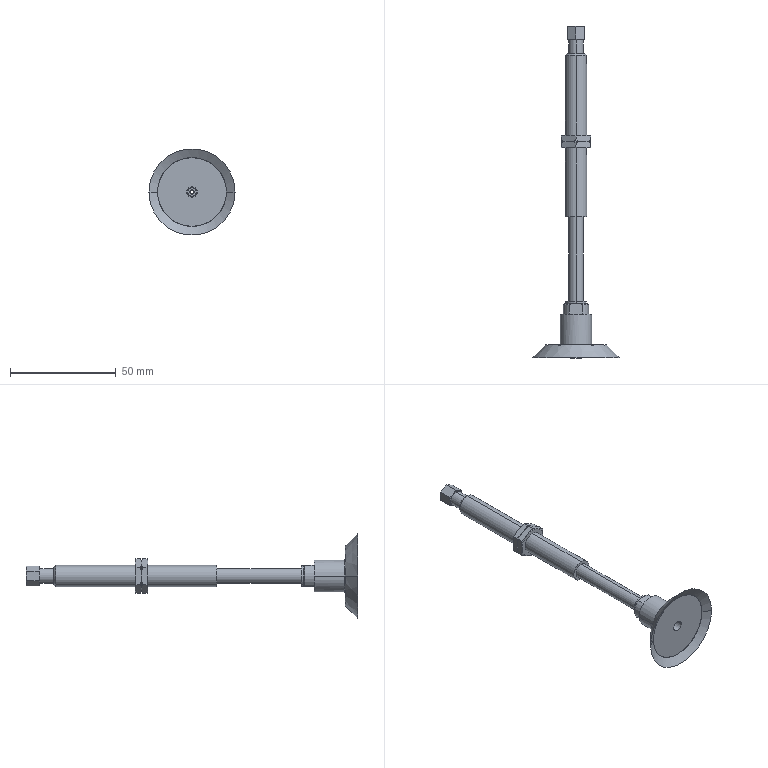Part | SolidWorks | features BaseBody 2 | 2 solids | 123 faces | box 40.704 x 156.673 x 40.704 mm | volume 14106 mm3 | cone 54 | plane 36 | cylinder 27 | torus 6 | commonest cylinder face diameters 5 x4 7 x4 10 x4 11.9 x3 2 x2 4.134 x2